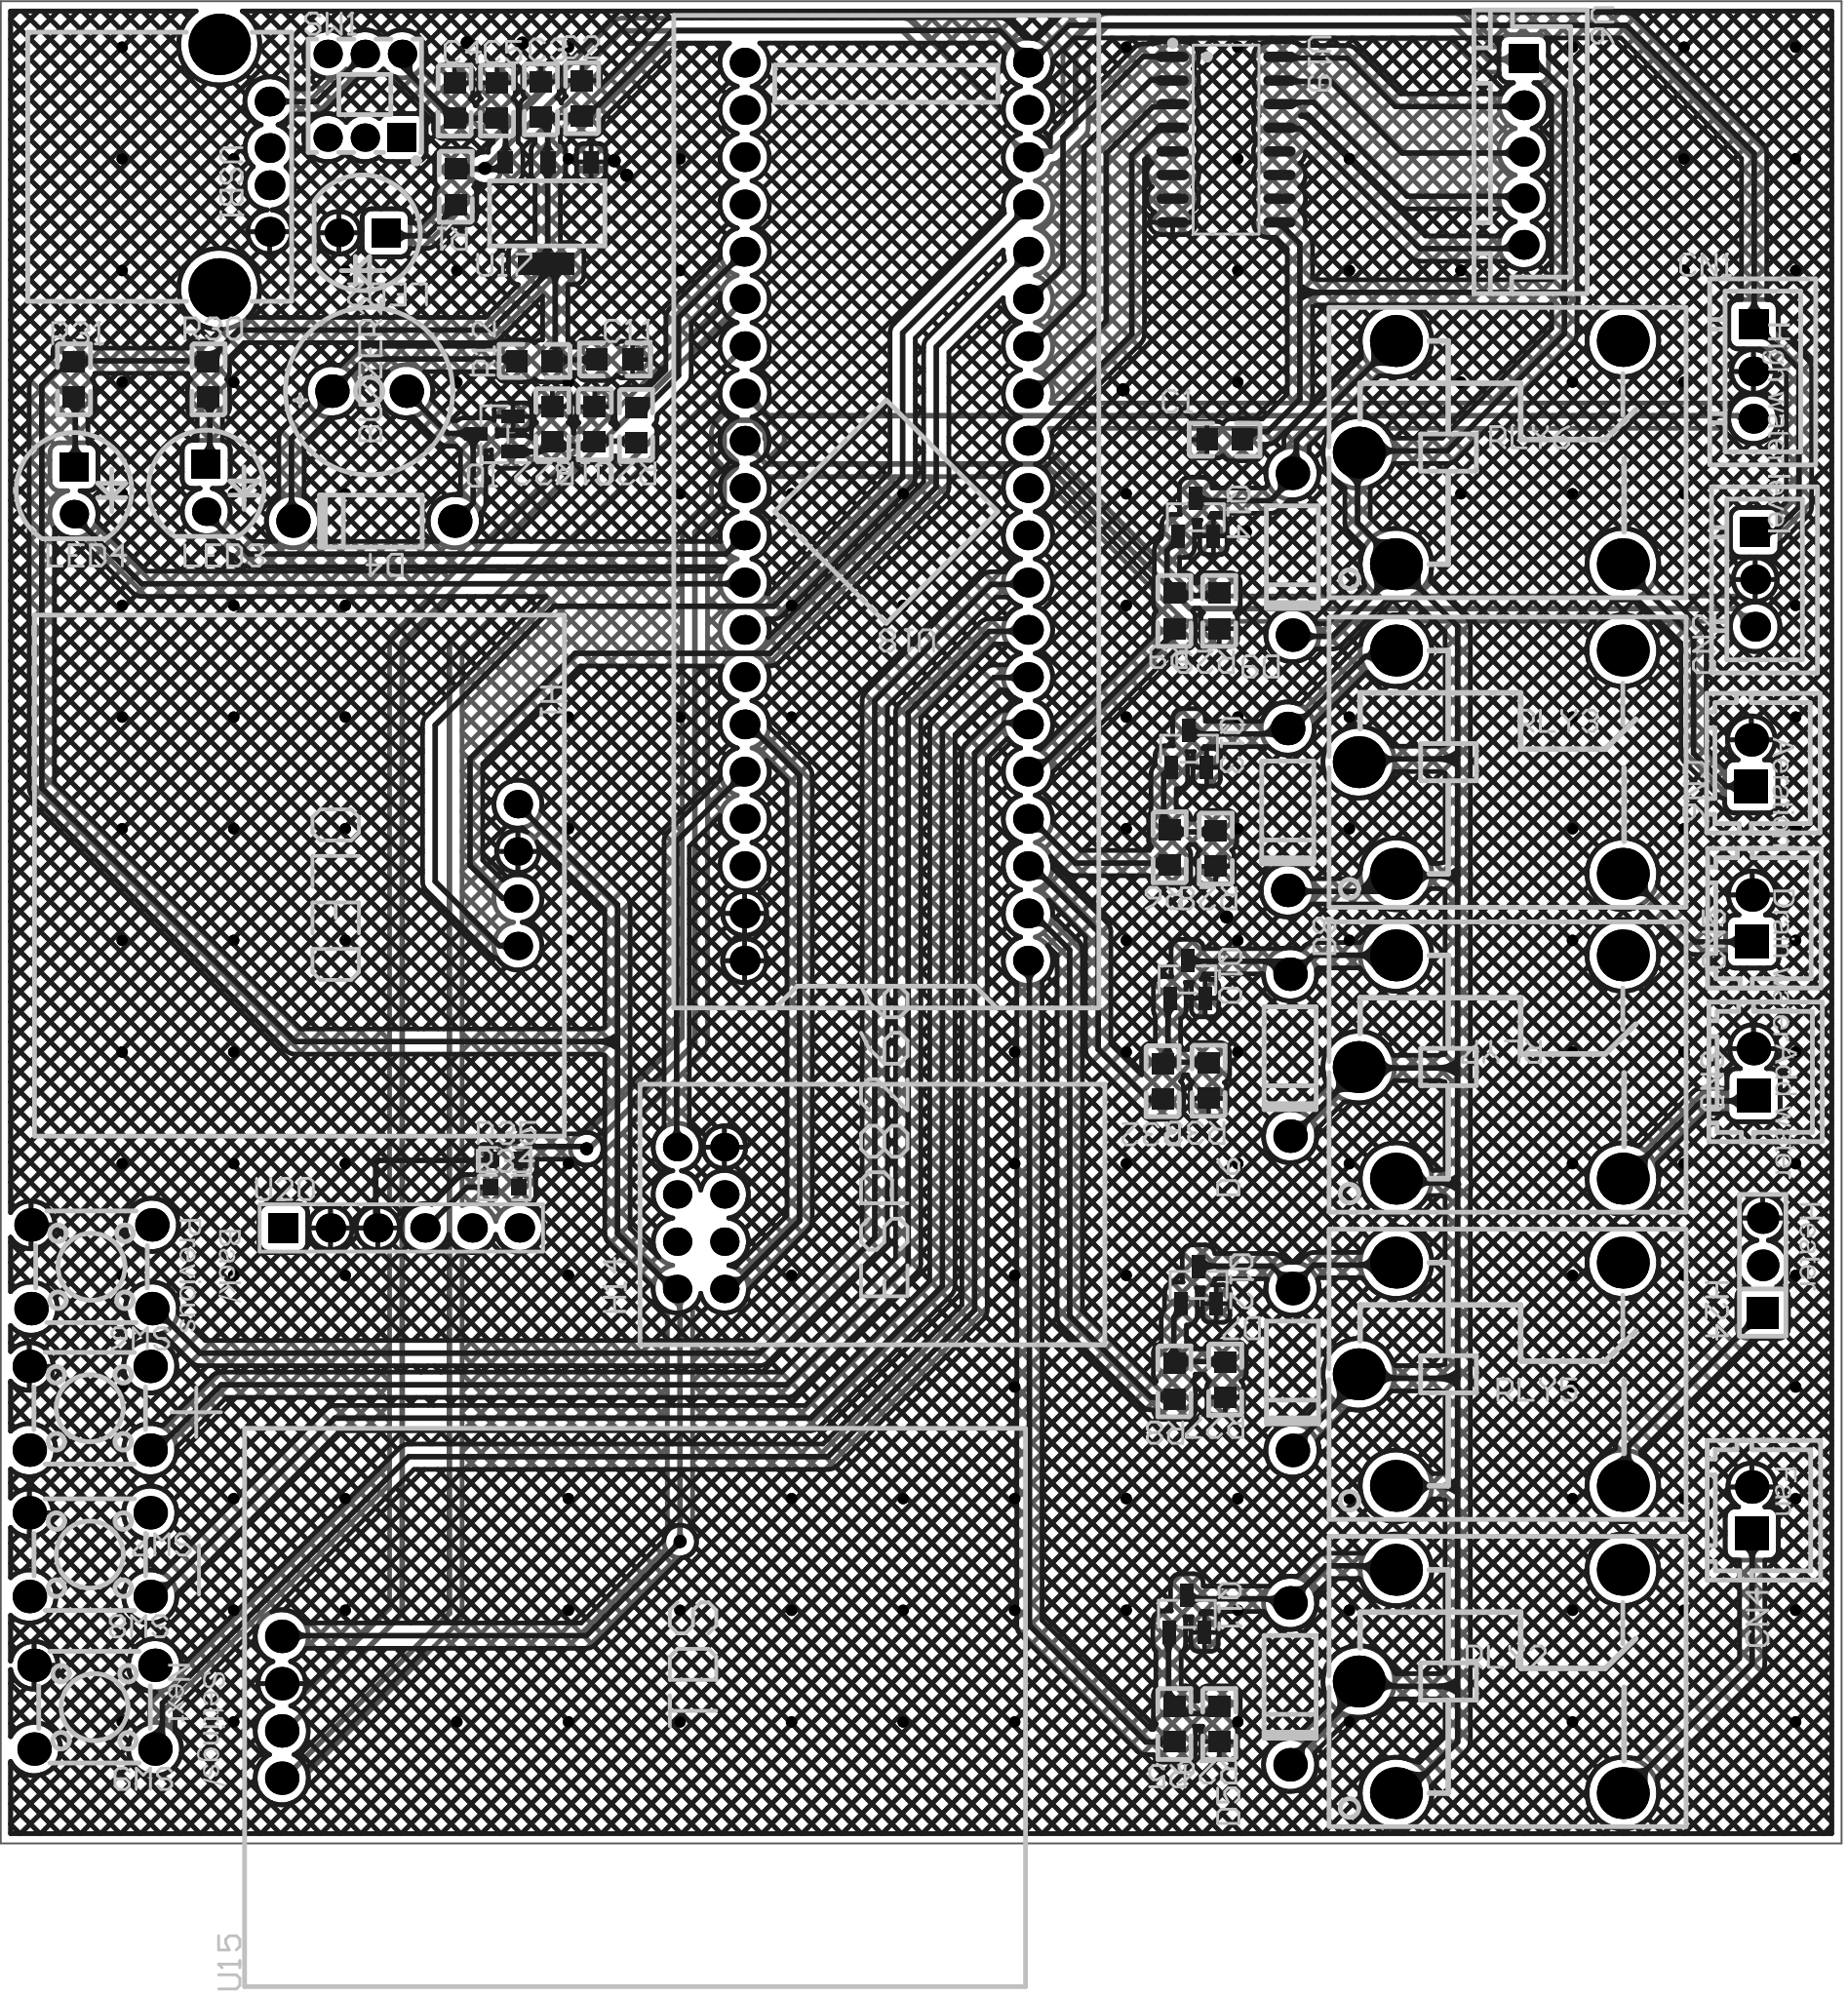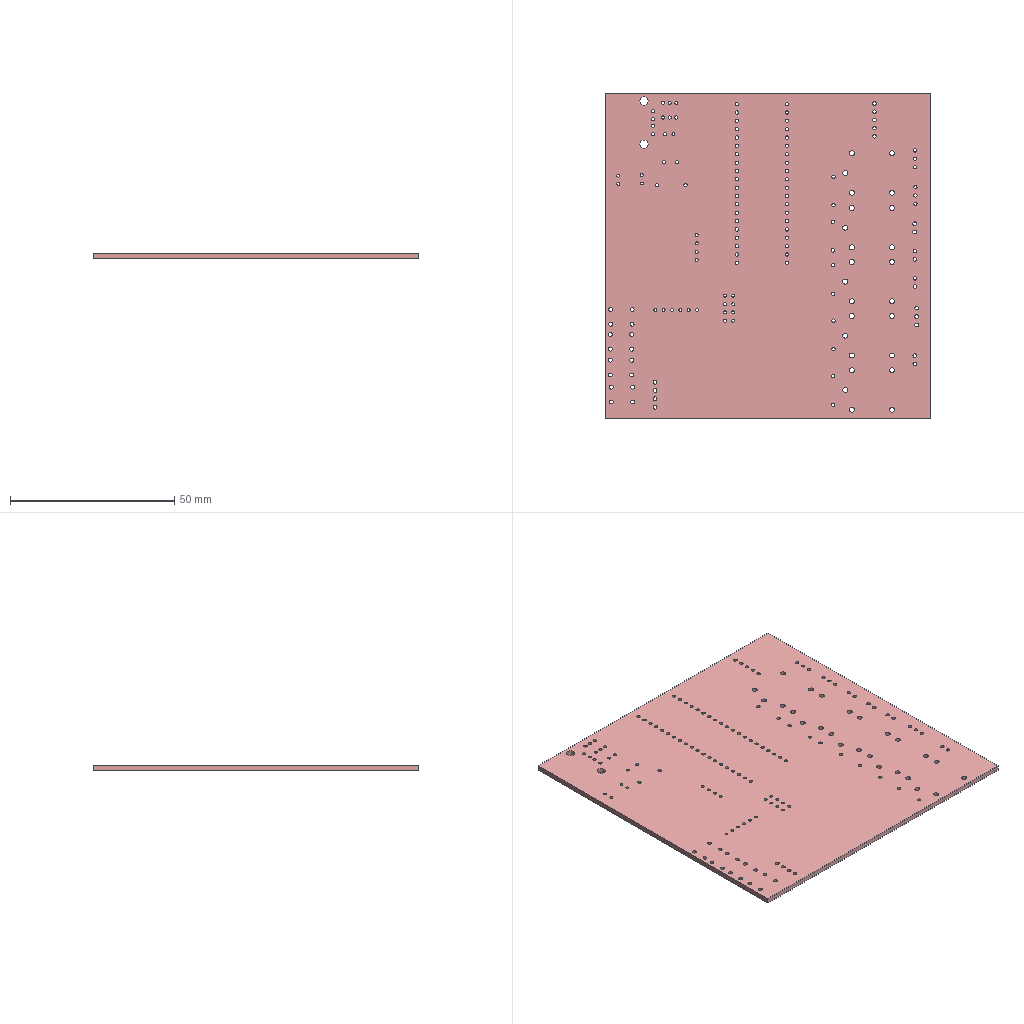Circuit board layout | Altium Designer | box 99 x 99 x 1.6 mm
Layer stack:
# Altium Designer layer stack of  (unit mm; dielectric type: 0 none, 1 core, 2 prepreg, 3 surface material)
index,name,kind,layer,copper_thickness_mm,dielectric_type,dielectric_thickness_mm,dielectric_material,dielectric_constant
0,Top Paste Mask Layer,other,,,,,,
1,Top Silkscreen Layer,other,,,,,,
2,Top Solder Mask Layer,dielectric,,,3,0.01,,3.3
3,Top Layer,copper,Top Layer,0.035,,,,
4,Dielectric1,dielectric,,,3,1.51,FR4,4.5
5,Bottom Layer,copper,Bottom Layer,0.035,,,,
6,Bottom Solder Mask Layer,dielectric,,,3,0.01,,3.3
7,Bottom Silkscreen Layer,other,,,,,,
8,Bottom Paste Mask Layer,other,,,,,,
# drill layer pairs: low layer,high layer
drill_pair,Top Layer,Bottom Layer
Part placement:
Designator,Comment,Layer,Footprint,Center-X(mm),Center-Y(mm),Rotation
CN1,ZX-XH2.54-3PZZ,TopLayer,CONN-TH_3P-P2.54_2501S-3P,173.956,162.994,270
R12,220,TopLayer,c0805,108.406,163.565,180
CN2,ZX-XH2.54-3PZZ,TopLayer,CONN-TH_3P-P2.54_2501S-3P,174.05,151.817,270
CN3,ZX-XH2.54-2PZZ,TopLayer,CONN-TH_2P-P2.50_HX25003-2A,173.961,125.357,90
SW1,5.8 ZSGT,TopLayer,SW-TH_5.8ZSGT,99.277,177.814,0
CN4,ZX-XH2.54-2PZZ,TopLayer,CONN-TH_2P-P2.50_HX25003-2A,173.867,101.799,90
U6,ZX-XH2.54-5PZZ,TopLayer,CONN-TH_5P-P2.50_ZX-XH2.54-5PZZ,161.602,174.802,270
R34,2.2K,TopLayer,R0603,106.782,119.138,0
CN5,ZX-XH2.54-2PZZ,TopLayer,CONN-TH_2P-P2.50_HX25003-2A,173.891,133.615,90
SW6,TS665CJ,TopLayer,SW-TH_4P-L6.0-W6.0-P4.50-LS6.5,84.575,114.883,180
SW7,TS665CJ,TopLayer,SW-TH_4P-L6.0-W6.0-P4.50-LS6.5,84.48,107.28,180
SW8,TS665CJ,TopLayer,SW-TH_4P-L6.0-W6.0-P4.50-LS6.5,84.484,99.414,180
SW9,TS665CJ,TopLayer,SW-TH_4P-L6.0-W6.0-P4.50-LS6.5,84.739,91.216,180
H1,OLED,TopLayer,oled,107.509,135.934,270
H24,Heater,TopLayer,HDR-TH_3P-P2.54-V-M,174.454,114.961,90
RLY2,SRD-05VDC-SL-C,TopLayer,RELAY-TH_SRD-XXVDC-XL-C,159.833,92.597,0
R5,,TopLayer,c0805,142.815,90.311,90
Q10,SS8050/SOT23-3,TopLayer,SOT-23-3_L2.9-W1.3-P1.90-LS2.4-BR,143.517,130.324,270
RLY3,SRD-05VDC-SL-C,TopLayer,RELAY-TH_SRD-XXVDC-XL-C,159.833,142,0
R6,,TopLayer,c0805,142.561,137.428,90
Q11,SS8050/SOT23-3,TopLayer,SOT-23-3_L2.9-W1.3-P1.90-LS2.4-BR,143.486,96.231,270
CN6,ZX-XH2.54-2PZZ,TopLayer,CONN-TH_2P-P2.50_HX25003-2A,173.843,141.95,90
Q12,SS8050/SOT23-3,TopLayer,SOT-23-3_L2.9-W1.3-P1.90-LS2.4-BR,144.116,113.905,270
Q13,SS8050/SOT23-3,TopLayer,SOT-23-3_L2.9-W1.3-P1.90-LS2.4-BR,143.603,142.722,270
RLY5,SRD-05VDC-SL-C,TopLayer,RELAY-TH_SRD-XXVDC-XL-C,159.833,109.107,0
R8,,TopLayer,c0805,142.815,108.726,90
Q14,SS8050/SOT23-3,TopLayer,SOT-23-3_L2.9-W1.3-P1.90-LS2.4-BR,143.965,155.161,270
U19,ULN2003A,TopLayer,SOP-16_L10.0-W3.9-P1.27-LS6.0-BL,145.594,175.457,270
R35,3.3K,TopLayer,R0603,106.835,120.636,0
U15,,TopLayer,TDS模块,94.809,91.21,90
RLY6,SRD-05VDC-SL-C,TopLayer,RELAY-TH_SRD-XXVDC-XL-C,159.833,158.637,0
R9,,TopLayer,c0805,142.815,150.128,90
U20,,TopLayer,HDR-M-2.54_1X6,101.239,116.969,0
H14,PZ254V-12-8P,TopLayer,esp8266,117.343,117.501,90
C11,104/0603,TopLayer,c0805,112.726,163.637,180
R22,10K/0603,TopLayer,c0805,109.361,160.162,270
C16,104/0603,TopLayer,c0805,111.644,160.149,270
U18,LCKFB-DKX-STM32F103C8T6,TopLayer,CONN-TH_L53.3-W22.9_STM32F103C8T6-CARD,127.321,155.462,90
BUZZER2,2.7kHz,TopLayer,BUZ-TH_BD9.0-P4.00-D0.6-FD,99.508,161.939,0
R26,10K/0603,TopLayer,c0805,145.228,90.311,90
R27,10K/0603,TopLayer,c0805,145.55,108.827,90
R28,10K/0603,TopLayer,c0805,145.04,137.357,90
R29,10K/0603,TopLayer,c0805,145.228,150.128,90
LED3,L-7113SGC,TopLayer,LED-TH_BD5.9-P2.54-FD,90.745,156.732,270
LED4,L-7113SGC,TopLayer,LED-TH_BD5.9-P2.54-FD,83.633,156.605,270
R30,,TopLayer,c0805,90.872,162.574,90
R31,,TopLayer,c0805,83.633,162.574,90
RLY7,SRD-05VDC-SL-C,TopLayer,RELAY-TH_SRD-XXVDC-XL-C,159.833,125.617,0
R32,,TopLayer,c0805,142.18,124.855,90
R33,10K/0603,TopLayer,c0805,144.654,124.879,90
C1,100nF,TopLayer,c0805,145.515,159.327,0
USB1,USB-231-ARY,TopLayer,USB-A-TH_USB-231-ARY,92.8,174.004,270
U17,AMS1117-3.3,TopLayer,sot-223,109.146,171.528,270
C5,0.1u,TopLayer,c0805,106.384,177.56,270
C2,0.1u,TopLayer,c0805,110.961,177.682,270
R1,,TopLayer,c0805,104.164,172.922,270
C3,10u,TopLayer,c0805,108.746,177.621,270
C4,10u,TopLayer,c0805,104.103,177.555,270
LED2,L-7113SGC,TopLayer,LED-TH_BD5.9-P2.54-FD,99.15,170.448,180
Q1,SS8050/SOT23-3,TopLayer,SOT-23-3_L2.9-W1.3-P1.90-LS2.4-BR,106.242,159.623,0
R20,1K/0603,TopLayer,c0805,113.862,160.126,270
D4,1N4007,TopLayer,DO-41_BD2.4-L4.7-P8.70-D0.8-RD,99.762,154.954,0
D5,1N4007,TopLayer,DO-41_BD2.4-L4.7-P8.70-D0.8-RD,149.038,92.47,90
D6,1N4007,TopLayer,DO-41_BD2.4-L4.7-P8.70-D0.8-RD,149.038,126.252,90
D7,1N4007,TopLayer,DO-41_BD2.4-L4.7-P8.70-D0.8-RD,149.165,109.361,90
D8,1N4007,TopLayer,DO-41_BD2.4-L4.7-P8.70-D0.8-RD,148.911,139.46,90
D9,1N4007,TopLayer,DO-41_BD2.4-L4.7-P8.70-D0.8-RD,149.165,153.176,90
Pad and via stacks:
# Altium Designer via and pad stacks of  (unit mm). Each distinct definition once, with the count of objects using it.
# via: kind,start_layer,end_layer,hole_mm,diameter_mm,mode(0 simple;1 top-mid-bottom;2 full stack),diameter_per_layer,count,example_net
# pad: kind,layer,hole_mm,hole_type(0 round;1 square;2 slot),plating,top_size,top_shape(1 round;2 rect;3 octagon;9 rounded rect),mid_size,bottom_size,mode,footprint,size_per_layer,count,example
pad,Multi-Layer,1,0,plated,1.6x1.6,2,1.6x1.6,1.6x1.6,0,CONN-TH_3P-P2.54_2501S-3P,,2,CN1.1
pad,Multi-Layer,1,0,plated,1.6x1.6,1,1.6x1.6,1.6x1.6,0,CONN-TH_3P-P2.54_2501S-3P,,4,CN1.2
pad,Multi-Layer,1.1,0,plated,1.8x1.8,2,1.8x1.8,1.8x1.8,0,CONN-TH_2P-P2.50_HX25003-2A,,4,CN3.1
pad,Multi-Layer,1.1,0,plated,1.8x1.8,1,1.8x1.8,1.8x1.8,0,CONN-TH_2P-P2.50_HX25003-2A,,4,CN3.2
pad,Multi-Layer,1,0,plated,1.524x1.524,1,1.524x1.524,1.524x1.524,0,SW-TH_5.8ZSGT,,5,SW1.4
pad,Multi-Layer,1,0,plated,1.524x1.524,2,1.524x1.524,1.524x1.524,0,SW-TH_5.8ZSGT,,1,SW1.1
pad,Multi-Layer,1.1,0,plated,1.6x1.6,1,1.6x1.6,1.6x1.6,0,CONN-TH_5P-P2.50_ZX-XH2.54-5PZZ,,4,U6.4
pad,Multi-Layer,1.1,0,plated,1.524x1.6,2,1.524x1.6,1.524x1.6,0,CONN-TH_5P-P2.50_ZX-XH2.54-5PZZ,,1,U6.1
pad,Multi-Layer,1.2,0,plated,1.8x1.8,1,1.8x1.8,1.8x1.8,0,SW-TH_4P-L6.0-W6.0-P4.50-LS6.5,,16,SW6.1
pad,Multi-Layer,0.9144,0,plated,1.524x1.524,1,1.524x1.524,1.524x1.524,0,oled,,4,H1.1
pad,Multi-Layer,1.1,0,plated,1.7x1.7,2,1.7x1.7,1.7x1.7,0,HDR-TH_3P-P2.54-V-M,,1,H24.1
pad,Multi-Layer,1.1,0,plated,1.7x1.7,1,1.7x1.7,1.7x1.7,0,HDR-TH_3P-P2.54-V-M,,2,H24.2
pad,Multi-Layer,1.524,0,plated,2.794x2.794,1,2.794x2.794,2.794x2.794,0,RELAY-TH_SRD-XXVDC-XL-C,,25,RLY2.2
pad,Multi-Layer,1.2,0,plated,1.8x1.8,1,1.8x1.8,1.8x1.8,0,TDS\u00C4\u00A3\u00BF\u00E9,,4,U15.1
pad,Multi-Layer,0.889,0,plated,1.575x1.575,1,1.575x1.575,1.575x1.575,0,HDR-M-2.54_1X6,,5,U20.6
pad,Multi-Layer,0.889,0,plated,1.575x1.575,2,1.575x1.575,1.575x1.575,0,HDR-M-2.54_1X6,,1,U20.1
pad,Multi-Layer,0.9144,0,plated,1.524x1.524,1,1.524x1.524,1.524x1.524,0,esp8266,,8,H14.1
pad,Multi-Layer,1,0,plated,1.6x1.6,1,1.6x1.6,1.6x1.6,0,CONN-TH_L53.3-W22.9_STM32F103C8T6-CARD,,40,U18.1
pad,Multi-Layer,1,0,plated,1.8x1.8,1,1.8x1.8,1.8x1.8,0,BUZ-TH_BD9.0-P4.00-D0.6-FD,,2,BUZZER2.1
pad,Multi-Layer,0.9144,0,plated,1.524x1.524,1,1.524x1.524,1.524x1.524,0,LED-TH_BD5.9-P2.54-FD,,3,LED3.2
pad,Multi-Layer,0.9144,0,plated,1.524x1.524,2,1.524x1.524,1.524x1.524,0,LED-TH_BD5.9-P2.54-FD,,3,LED3.1
pad,Multi-Layer,1,0,plated,1.6x1.6,1,1.6x1.6,1.6x1.6,0,USB-A-TH_USB-231-ARY,,4,USB1.1
pad,Multi-Layer,2.5,0,plated,3.3x3.3,1,3.3x3.3,3.3x3.3,0,USB-A-TH_USB-231-ARY,,2,USB1.5
pad,Multi-Layer,1.05,0,plated,1.8x1.8,1,1.8x1.8,1.8x1.8,0,DO-41_BD2.4-L4.7-P8.70-D0.8-RD,,12,D4.2
pad,Top Layer,0,0,plated,1.14x1.2,2,1.14x1.2,1.14x1.2,0,c0805,,46,R12.1
pad,Top Layer,0,0,plated,0.8065x0.864,2,0.8065x0.864,0.8065x0.864,0,R0603,,4,R34.2
pad,Top Layer,0,0,plated,1.25x0.7,2,1.25x0.7,1.25x0.7,0,SOT-23-3_L2.9-W1.3-P1.90-LS2.4-BR,,18,Q10.1
pad,Top Layer,0,0,plated,0.56x1.745,1,0.56x1.745,0.56x1.745,0,SOP-16_L10.0-W3.9-P1.27-LS6.0-BL,,16,U19.1
pad,Top Layer,0,0,plated,1.2x0.8,2,1.2x0.8,1.2x0.8,0,sot-223,,3,U17.1
pad,Top Layer,0,0,plated,1.2x3,2,1.2x3,1.2x3,0,sot-223,,1,U17.4
via,Top Layer,Bottom Layer,0.5004,0.7,0,,10,5V
via,Top Layer,Bottom Layer,0.3048,0.61,0,,149,GND
Copper pours:
name,layer,net,type(0 solid;1 hatched;2 none)
Top Layer-GND,Top Layer,GND,0
Bottom Layer-GND,Bottom Layer,GND,0
Design rules, without the lines most boards share:
# Altium Designer design rules of  (exported by Altium Designer, unit mm)
# columns: name | kind | enabled | priority | scope1 | scope2 | descriptor | typed fields (field=value)
Copper_copperRegion1 | 0 | disabled | 4 | All | All | Clearance Constraint (Gap=5.984mil) (Disabled)(All),(All) | gap=0.152
Copper_copperRegion1_1 | 63 | disabled | 4 | All | All | Board Clearance Constraint (Gap=0mil) (Disabled)(All) |
copperThickness1oz | 0 | enabled | 5 | All | All | Clearance Constraint (Gap=5.984mil) (All),(All) | gap=0.152
copperThickness1oz_1 | 63 | enabled | 5 | All | All | Board Clearance Constraint (Gap=0mil) (All) |
otherClearance | 52 | enabled | 1 | All | All | Hole To Hole Clearance (Gap=11.8mil) (All),(All) | gap=0.2997
copperRegion1 | 20 | disabled | 1 | All | All | Polygon Connect Rule(Relief Connect )(Conductor Width=10mil) (Relief Angle=90 Angle) (Entries=4) (Air Gap Width=10mil) (Disabled)(All),(All) | connect_style(0=relief,1=direct,2=none)=0 relief_conductor_width=0.254 relief_entries=4
copperRegion | 20 | enabled | 2 | All | All | Polygon Connect Rule(Relief Connect )(Conductor Width=10mil) (Relief Angle=90 Angle) (Entries=4) (Air Gap Width=10mil) (All),(All) | connect_style(0=relief,1=direct,2=none)=0 relief_conductor_width=0.254 relief_entries=4
solderMaskExpansion | 13 | enabled | 2 | All | All | Solder Mask Expansion (Expansion =2.008mil) (All) | expansion=0.051